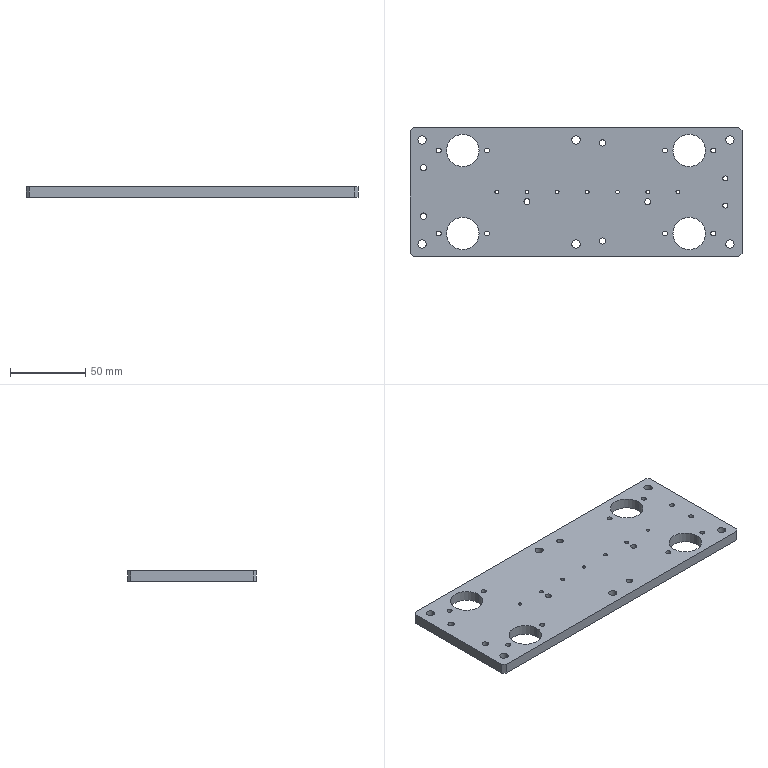Part | STEP file | PN_0007 | 1 solid | 76 faces | box 220 x 85 x 7 mm | volume 118278 mm3 | cylinder 66 | plane 10 | commonest cylinder face diameters 3.3 x20 2.5 x14 5.5 x12 4.2 x8 21.5 x8 4 x4